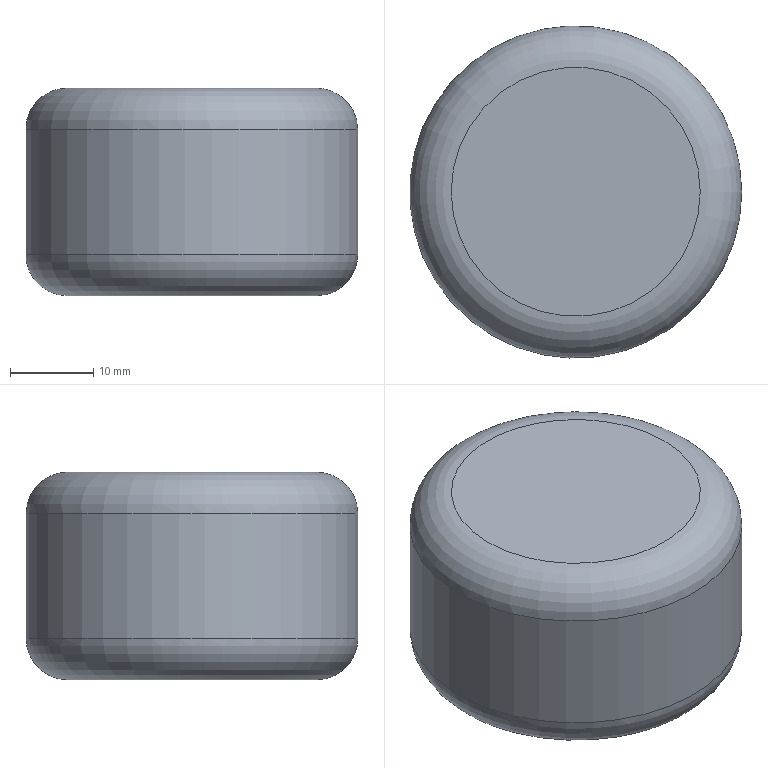Part | NX | features DATUM_CSYS 2, BLEND 1, EXTRUDE 1, SKETCH 1 | 1 solid | 5 faces | box 40 x 40 x 25 mm | volume 30143 mm3 | plane 2 | torus 2 | cylinder 1 | commonest cylinder face diameters 40 x1
STEP:
#1=CARTESIAN_POINT('',(20.,0.,5.));
#2=VERTEX_POINT('',#1);
#3=CARTESIAN_POINT('',(0.,0.,5.));
#4=DIRECTION('',(0.,0.,1.));
#5=DIRECTION('',(1.,0.,0.));
#6=AXIS2_PLACEMENT_3D('',#3,#4,#5);
#7=CIRCLE('',#6,20.);
#8=EDGE_CURVE('',#2,#2,#7,.T.);
#9=ORIENTED_EDGE('',*,*,#8,.T.);
#10=EDGE_LOOP('',(#9));
#11=FACE_BOUND('',#10,.T.);
#12=CARTESIAN_POINT('',(20.,0.,20.));
#13=VERTEX_POINT('',#12);
#14=CARTESIAN_POINT('',(0.,0.,20.));
#15=DIRECTION('',(0.,0.,1.));
#16=DIRECTION('',(1.,0.,0.));
#17=AXIS2_PLACEMENT_3D('',#14,#15,#16);
#18=CIRCLE('',#17,20.);
#19=EDGE_CURVE('',#13,#13,#18,.F.);
#20=ORIENTED_EDGE('',*,*,#19,.T.);
#21=EDGE_LOOP('',(#20));
#22=FACE_BOUND('',#21,.T.);
#23=CARTESIAN_POINT('',(0.,0.,25.));
#24=DIRECTION('',(0.,0.,-1.));
#25=DIRECTION('',(-1.,0.,0.));
#26=AXIS2_PLACEMENT_3D('',#23,#24,#25);
#27=CYLINDRICAL_SURFACE('',#26,20.);
#28=ADVANCED_FACE('',(#11,#22),#27,.T.);
#29=CARTESIAN_POINT('',(15.,0.,25.));
#30=VERTEX_POINT('',#29);
#31=CARTESIAN_POINT('',(0.,0.,25.));
#32=DIRECTION('',(0.,0.,1.));
#33=DIRECTION('',(1.,0.,0.));
#34=AXIS2_PLACEMENT_3D('',#31,#32,#33);
#35=CIRCLE('',#34,15.);
#36=EDGE_CURVE('',#30,#30,#35,.T.);
#37=ORIENTED_EDGE('',*,*,#36,.T.);
#38=EDGE_LOOP('',(#37));
#39=FACE_BOUND('',#38,.T.);
#40=CARTESIAN_POINT('',(0.,0.,25.));
#41=DIRECTION('',(0.,0.,1.));
#42=DIRECTION('',(1.,0.,0.));
#43=AXIS2_PLACEMENT_3D('',#40,#41,#42);
#44=PLANE('',#43);
#45=ADVANCED_FACE('',(#39),#44,.T.);
#46=CARTESIAN_POINT('',(15.,0.,0.));
#47=VERTEX_POINT('',#46);
#48=CARTESIAN_POINT('',(0.,0.,0.));
#49=DIRECTION('',(0.,0.,1.));
#50=DIRECTION('',(1.,0.,0.));
#51=AXIS2_PLACEMENT_3D('',#48,#49,#50);
#52=CIRCLE('',#51,15.);
#53=EDGE_CURVE('',#47,#47,#52,.F.);
#54=ORIENTED_EDGE('',*,*,#53,.T.);
#55=EDGE_LOOP('',(#54));
#56=FACE_BOUND('',#55,.T.);
#57=CARTESIAN_POINT('',(0.,0.,0.));
#58=DIRECTION('',(0.,0.,1.));
#59=DIRECTION('',(1.,0.,0.));
#60=AXIS2_PLACEMENT_3D('',#57,#58,#59);
#61=PLANE('',#60);
#62=ADVANCED_FACE('',(#56),#61,.F.);
#63=ORIENTED_EDGE('',*,*,#53,.F.);
#64=EDGE_LOOP('',(#63));
#65=FACE_BOUND('',#64,.T.);
#66=ORIENTED_EDGE('',*,*,#8,.F.);
#67=EDGE_LOOP('',(#66));
#68=FACE_BOUND('',#67,.T.);
#69=CARTESIAN_POINT('',(0.,0.,5.));
#70=DIRECTION('',(0.,0.,1.));
#71=DIRECTION('',(1.,0.,0.));
#72=AXIS2_PLACEMENT_3D('',#69,#70,#71);
#73=TOROIDAL_SURFACE('',#72,15.,5.);
#74=ADVANCED_FACE('',(#65,#68),#73,.T.);
#75=ORIENTED_EDGE('',*,*,#19,.F.);
#76=EDGE_LOOP('',(#75));
#77=FACE_BOUND('',#76,.T.);
#78=ORIENTED_EDGE('',*,*,#36,.F.);
#79=EDGE_LOOP('',(#78));
#80=FACE_BOUND('',#79,.T.);
#81=CARTESIAN_POINT('',(0.,0.,20.));
#82=DIRECTION('',(0.,0.,1.));
#83=DIRECTION('',(1.,0.,0.));
#84=AXIS2_PLACEMENT_3D('',#81,#82,#83);
#85=TOROIDAL_SURFACE('',#84,15.,5.);
#86=ADVANCED_FACE('',(#77,#80),#85,.T.);
#87=CLOSED_SHELL('',(#28,#45,#62,#74,#86));
#88=MANIFOLD_SOLID_BREP('',#87);
#89=(LENGTH_UNIT()NAMED_UNIT(*)SI_UNIT(.MILLI.,.METRE.));
#90=UNCERTAINTY_MEASURE_WITH_UNIT(LENGTH_MEASURE(0.00001),#89,'','');
#91=(NAMED_UNIT(*)PLANE_ANGLE_UNIT()SI_UNIT($,.RADIAN.));
#92=(NAMED_UNIT(*)SI_UNIT($,.STERADIAN.)SOLID_ANGLE_UNIT());
#93=(GEOMETRIC_REPRESENTATION_CONTEXT(3)GLOBAL_UNCERTAINTY_ASSIGNED_CONTEXT((#90))GLOBAL_UNIT_ASSIGNED_CONTEXT((#89,#91,#92))REPRESENTATION_CONTEXT('',''));
#94=ADVANCED_BREP_SHAPE_REPRESENTATION('',(#88),#93);